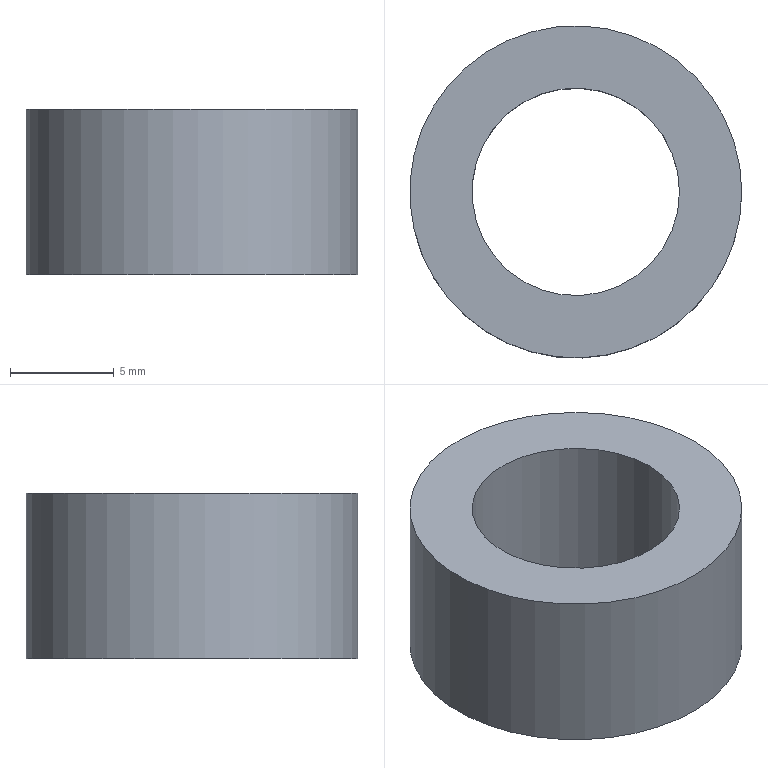Part | NX | features BREP 1 | 1 solid | 4 faces | box 16 x 16 x 8 mm | volume 980.177 mm3 | cylinder 2 | plane 2 | commonest cylinder face diameters 10 x1 16 x1
STEP:
#1=CARTESIAN_POINT('',(5.,0.,-4.));
#2=VERTEX_POINT('',#1);
#3=CARTESIAN_POINT('',(0.,0.,-4.));
#4=DIRECTION('',(0.,0.,1.));
#5=DIRECTION('',(1.,0.,0.));
#6=AXIS2_PLACEMENT_3D('',#3,#4,#5);
#7=CIRCLE('',#6,5.);
#8=EDGE_CURVE('',#2,#2,#7,.T.);
#9=ORIENTED_EDGE('',*,*,#8,.F.);
#10=EDGE_LOOP('',(#9));
#11=FACE_BOUND('',#10,.T.);
#12=CARTESIAN_POINT('',(5.,0.,4.));
#13=VERTEX_POINT('',#12);
#14=CARTESIAN_POINT('',(0.,0.,4.));
#15=DIRECTION('',(0.,0.,1.));
#16=DIRECTION('',(1.,0.,0.));
#17=AXIS2_PLACEMENT_3D('',#14,#15,#16);
#18=CIRCLE('',#17,5.);
#19=EDGE_CURVE('',#13,#13,#18,.T.);
#20=ORIENTED_EDGE('',*,*,#19,.T.);
#21=EDGE_LOOP('',(#20));
#22=FACE_BOUND('',#21,.T.);
#23=CARTESIAN_POINT('',(0.,0.,4.));
#24=DIRECTION('',(0.,0.,1.));
#25=DIRECTION('',(-1.,0.,0.));
#26=AXIS2_PLACEMENT_3D('',#23,#24,#25);
#27=CYLINDRICAL_SURFACE('',#26,5.);
#28=ADVANCED_FACE('',(#11,#22),#27,.F.);
#29=CARTESIAN_POINT('',(8.,0.,-4.));
#30=VERTEX_POINT('',#29);
#31=CARTESIAN_POINT('',(0.,0.,-4.));
#32=DIRECTION('',(0.,0.,1.));
#33=DIRECTION('',(1.,0.,0.));
#34=AXIS2_PLACEMENT_3D('',#31,#32,#33);
#35=CIRCLE('',#34,8.);
#36=EDGE_CURVE('',#30,#30,#35,.T.);
#37=ORIENTED_EDGE('',*,*,#36,.T.);
#38=EDGE_LOOP('',(#37));
#39=FACE_BOUND('',#38,.T.);
#40=CARTESIAN_POINT('',(8.,0.,4.));
#41=VERTEX_POINT('',#40);
#42=CARTESIAN_POINT('',(0.,0.,4.));
#43=DIRECTION('',(0.,0.,1.));
#44=DIRECTION('',(1.,0.,0.));
#45=AXIS2_PLACEMENT_3D('',#42,#43,#44);
#46=CIRCLE('',#45,8.);
#47=EDGE_CURVE('',#41,#41,#46,.T.);
#48=ORIENTED_EDGE('',*,*,#47,.F.);
#49=EDGE_LOOP('',(#48));
#50=FACE_BOUND('',#49,.T.);
#51=CARTESIAN_POINT('',(0.,0.,4.));
#52=DIRECTION('',(0.,0.,1.));
#53=DIRECTION('',(-1.,0.,0.));
#54=AXIS2_PLACEMENT_3D('',#51,#52,#53);
#55=CYLINDRICAL_SURFACE('',#54,8.);
#56=ADVANCED_FACE('',(#39,#50),#55,.T.);
#57=ORIENTED_EDGE('',*,*,#36,.F.);
#58=EDGE_LOOP('',(#57));
#59=FACE_BOUND('',#58,.T.);
#60=ORIENTED_EDGE('',*,*,#8,.T.);
#61=EDGE_LOOP('',(#60));
#62=FACE_BOUND('',#61,.T.);
#63=CARTESIAN_POINT('',(0.,0.,-4.));
#64=DIRECTION('',(0.,0.,1.));
#65=DIRECTION('',(1.,0.,0.));
#66=AXIS2_PLACEMENT_3D('',#63,#64,#65);
#67=PLANE('',#66);
#68=ADVANCED_FACE('',(#59,#62),#67,.F.);
#69=ORIENTED_EDGE('',*,*,#47,.T.);
#70=EDGE_LOOP('',(#69));
#71=FACE_BOUND('',#70,.T.);
#72=ORIENTED_EDGE('',*,*,#19,.F.);
#73=EDGE_LOOP('',(#72));
#74=FACE_BOUND('',#73,.T.);
#75=CARTESIAN_POINT('',(0.,0.,4.));
#76=DIRECTION('',(0.,0.,1.));
#77=DIRECTION('',(1.,0.,0.));
#78=AXIS2_PLACEMENT_3D('',#75,#76,#77);
#79=PLANE('',#78);
#80=ADVANCED_FACE('',(#71,#74),#79,.T.);
#81=CLOSED_SHELL('',(#28,#56,#68,#80));
#82=MANIFOLD_SOLID_BREP('',#81);
#83=(LENGTH_UNIT()NAMED_UNIT(*)SI_UNIT(.MILLI.,.METRE.));
#84=UNCERTAINTY_MEASURE_WITH_UNIT(LENGTH_MEASURE(0.00001),#83,'','');
#85=(NAMED_UNIT(*)PLANE_ANGLE_UNIT()SI_UNIT($,.RADIAN.));
#86=(NAMED_UNIT(*)SI_UNIT($,.STERADIAN.)SOLID_ANGLE_UNIT());
#87=(GEOMETRIC_REPRESENTATION_CONTEXT(3)GLOBAL_UNCERTAINTY_ASSIGNED_CONTEXT((#84))GLOBAL_UNIT_ASSIGNED_CONTEXT((#83,#85,#86))REPRESENTATION_CONTEXT('',''));
#88=ADVANCED_BREP_SHAPE_REPRESENTATION('',(#82),#87);